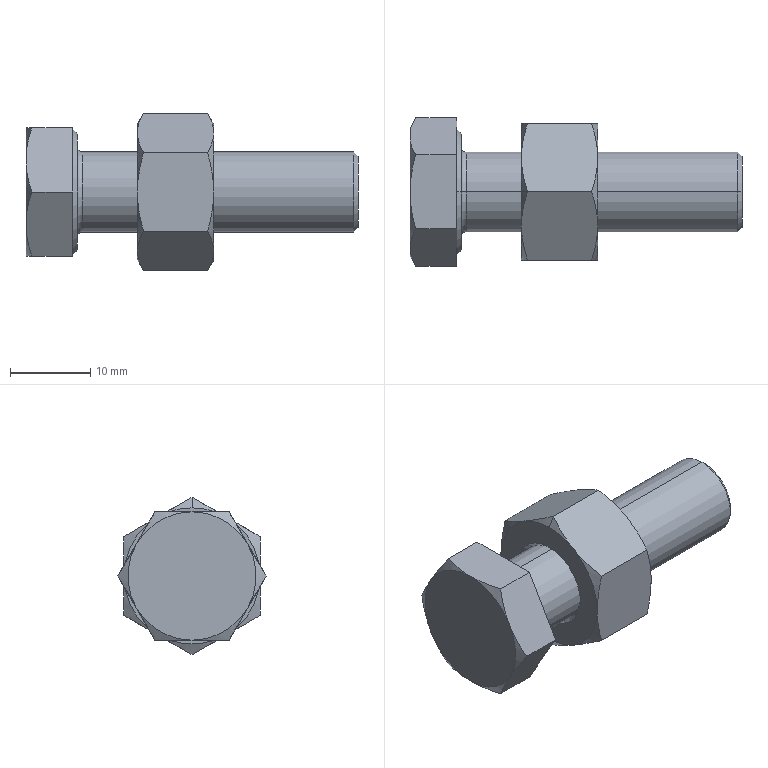Part | SolidWorks | features BaseBody 2 | 2 solids | 52 faces | box 41.4 x 18.475 x 19.63 mm | volume 5747 mm3 | cone 28 | plane 18 | cylinder 4 | torus 2 | commonest cylinder face diameters 10 x4